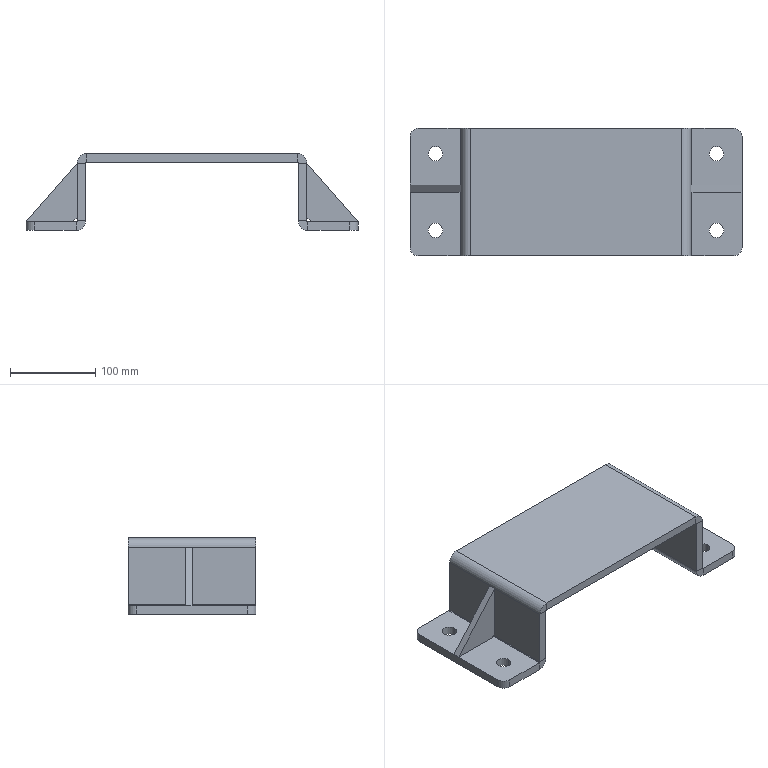Part | SolidWorks | 3 solids | 62 faces | box 390 x 150 x 90 mm | volume 832531 mm3 | plane 42 | cylinder 20 | commonest cylinder face diameters 17 x8 2 x4 20 x4 22 x4